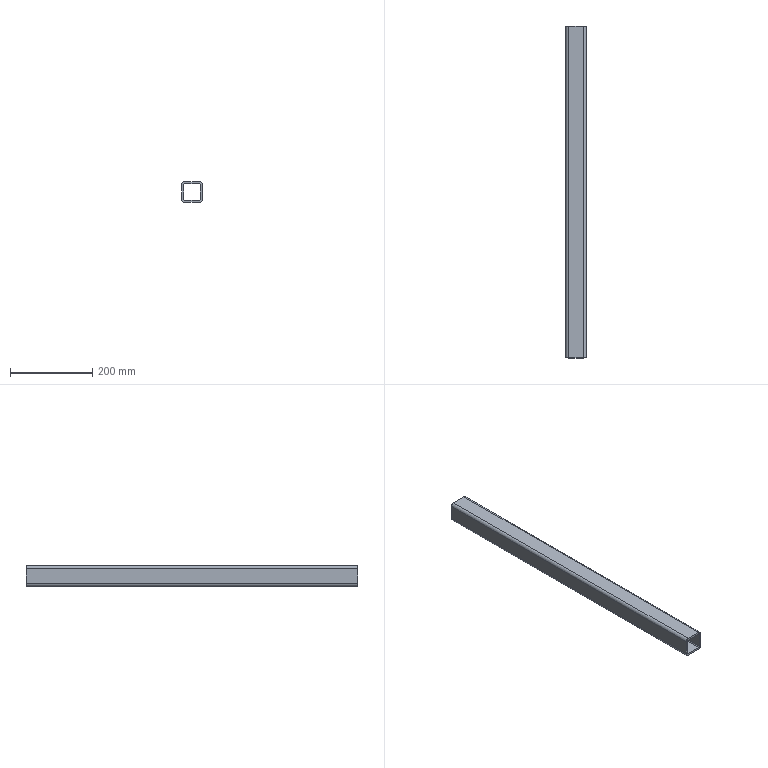Part | NX | 1 solid | 21 faces | box 50 x 806 x 50 mm | volume 694058 mm3 | cylinder 11 | plane 10 | commonest cylinder face diameters 4 x4 14 x4 4.2 x3
STEP:
#1=CARTESIAN_POINT('',(-895.,25.,-328.));
#2=VERTEX_POINT('',#1);
#3=CARTESIAN_POINT('',(-895.,831.,-328.));
#4=VERTEX_POINT('',#3);
#5=CARTESIAN_POINT('',(-895.,0.,-328.));
#6=DIRECTION('',(0.,1.,0.));
#7=VECTOR('',#6,1000.);
#8=LINE('',#5,#7);
#9=EDGE_CURVE('',#2,#4,#8,.T.);
#10=ORIENTED_EDGE('',*,*,#9,.T.);
#11=CARTESIAN_POINT('',(-895.,831.,-292.));
#12=VERTEX_POINT('',#11);
#13=CARTESIAN_POINT('',(-895.,831.,-328.));
#14=DIRECTION('',(0.,0.,1.));
#15=VECTOR('',#14,1000.);
#16=LINE('',#13,#15);
#17=EDGE_CURVE('',#4,#12,#16,.T.);
#18=ORIENTED_EDGE('',*,*,#17,.T.);
#19=CARTESIAN_POINT('',(-895.,25.,-292.));
#20=VERTEX_POINT('',#19);
#21=CARTESIAN_POINT('',(-895.,0.,-292.));
#22=DIRECTION('',(0.,1.,0.));
#23=VECTOR('',#22,1000.);
#24=LINE('',#21,#23);
#25=EDGE_CURVE('',#20,#12,#24,.T.);
#26=ORIENTED_EDGE('',*,*,#25,.F.);
#27=CARTESIAN_POINT('',(-895.,25.,-328.));
#28=DIRECTION('',(0.,0.,-1.));
#29=VECTOR('',#28,1000.);
#30=LINE('',#27,#29);
#31=EDGE_CURVE('',#20,#2,#30,.T.);
#32=ORIENTED_EDGE('',*,*,#31,.T.);
#33=EDGE_LOOP('',(#10,#18,#26,#32));
#34=FACE_BOUND('',#33,.T.);
#35=CARTESIAN_POINT('',(-895.,0.,-328.));
#36=DIRECTION('',(1.,0.,0.));
#37=DIRECTION('',(0.,0.,-1.));
#38=AXIS2_PLACEMENT_3D('',#35,#36,#37);
#39=PLANE('',#38);
#40=ADVANCED_FACE('',(#34),#39,.T.);
#41=CARTESIAN_POINT('',(-893.,25.,-330.));
#42=VERTEX_POINT('',#41);
#43=CARTESIAN_POINT('',(-893.,831.,-330.));
#44=VERTEX_POINT('',#43);
#45=CARTESIAN_POINT('',(-893.,0.,-330.));
#46=DIRECTION('',(0.,1.,0.));
#47=VECTOR('',#46,1000.);
#48=LINE('',#45,#47);
#49=EDGE_CURVE('',#42,#44,#48,.T.);
#50=ORIENTED_EDGE('',*,*,#49,.T.);
#51=CARTESIAN_POINT('',(-893.,831.,-328.));
#52=DIRECTION('',(0.,1.,0.));
#53=DIRECTION('',(-1.,0.,0.));
#54=AXIS2_PLACEMENT_3D('',#51,#52,#53);
#55=CIRCLE('',#54,2.);
#56=EDGE_CURVE('',#44,#4,#55,.T.);
#57=ORIENTED_EDGE('',*,*,#56,.T.);
#58=ORIENTED_EDGE('',*,*,#9,.F.);
#59=CARTESIAN_POINT('',(-893.,25.,-328.));
#60=DIRECTION('',(0.,-1.,0.));
#61=DIRECTION('',(1.,0.,0.));
#62=AXIS2_PLACEMENT_3D('',#59,#60,#61);
#63=CIRCLE('',#62,2.);
#64=EDGE_CURVE('',#2,#42,#63,.T.);
#65=ORIENTED_EDGE('',*,*,#64,.T.);
#66=EDGE_LOOP('',(#50,#57,#58,#65));
#67=FACE_BOUND('',#66,.T.);
#68=CARTESIAN_POINT('',(-893.,0.,-328.));
#69=DIRECTION('',(0.,1.,0.));
#70=DIRECTION('',(0.,0.,1.));
#71=AXIS2_PLACEMENT_3D('',#68,#69,#70);
#72=CYLINDRICAL_SURFACE('',#71,2.);
#73=ADVANCED_FACE('',(#67),#72,.F.);
#74=CARTESIAN_POINT('',(-857.,25.,-330.));
#75=VERTEX_POINT('',#74);
#76=CARTESIAN_POINT('',(-857.,831.,-330.));
#77=VERTEX_POINT('',#76);
#78=CARTESIAN_POINT('',(-857.,0.,-330.));
#79=DIRECTION('',(0.,1.,0.));
#80=VECTOR('',#79,1000.);
#81=LINE('',#78,#80);
#82=EDGE_CURVE('',#75,#77,#81,.T.);
#83=ORIENTED_EDGE('',*,*,#82,.T.);
#84=CARTESIAN_POINT('',(-893.,831.,-330.));
#85=DIRECTION('',(-1.,0.,0.));
#86=VECTOR('',#85,1000.);
#87=LINE('',#84,#86);
#88=EDGE_CURVE('',#77,#44,#87,.T.);
#89=ORIENTED_EDGE('',*,*,#88,.T.);
#90=ORIENTED_EDGE('',*,*,#49,.F.);
#91=CARTESIAN_POINT('',(-893.,25.,-330.));
#92=DIRECTION('',(1.,0.,0.));
#93=VECTOR('',#92,1000.);
#94=LINE('',#91,#93);
#95=EDGE_CURVE('',#42,#75,#94,.T.);
#96=ORIENTED_EDGE('',*,*,#95,.T.);
#97=EDGE_LOOP('',(#83,#89,#90,#96));
#98=FACE_BOUND('',#97,.T.);
#99=CARTESIAN_POINT('',(-893.,0.,-330.));
#100=DIRECTION('',(0.,0.,1.));
#101=DIRECTION('',(1.,0.,0.));
#102=AXIS2_PLACEMENT_3D('',#99,#100,#101);
#103=PLANE('',#102);
#104=ADVANCED_FACE('',(#98),#103,.T.);
#105=CARTESIAN_POINT('',(-855.,25.,-328.));
#106=VERTEX_POINT('',#105);
#107=CARTESIAN_POINT('',(-855.,831.,-328.));
#108=VERTEX_POINT('',#107);
#109=CARTESIAN_POINT('',(-855.,0.,-328.));
#110=DIRECTION('',(0.,1.,0.));
#111=VECTOR('',#110,1000.);
#112=LINE('',#109,#111);
#113=EDGE_CURVE('',#106,#108,#112,.T.);
#114=ORIENTED_EDGE('',*,*,#113,.T.);
#115=CARTESIAN_POINT('',(-857.,831.,-328.));
#116=DIRECTION('',(0.,1.,0.));
#117=DIRECTION('',(-1.,0.,0.));
#118=AXIS2_PLACEMENT_3D('',#115,#116,#117);
#119=CIRCLE('',#118,2.);
#120=EDGE_CURVE('',#108,#77,#119,.T.);
#121=ORIENTED_EDGE('',*,*,#120,.T.);
#122=ORIENTED_EDGE('',*,*,#82,.F.);
#123=CARTESIAN_POINT('',(-857.,25.,-328.));
#124=DIRECTION('',(0.,-1.,0.));
#125=DIRECTION('',(1.,0.,0.));
#126=AXIS2_PLACEMENT_3D('',#123,#124,#125);
#127=CIRCLE('',#126,2.);
#128=EDGE_CURVE('',#75,#106,#127,.T.);
#129=ORIENTED_EDGE('',*,*,#128,.T.);
#130=EDGE_LOOP('',(#114,#121,#122,#129));
#131=FACE_BOUND('',#130,.T.);
#132=CARTESIAN_POINT('',(-857.,0.,-328.));
#133=DIRECTION('',(0.,1.,0.));
#134=DIRECTION('',(0.,0.,1.));
#135=AXIS2_PLACEMENT_3D('',#132,#133,#134);
#136=CYLINDRICAL_SURFACE('',#135,2.);
#137=ADVANCED_FACE('',(#131),#136,.F.);
#138=CARTESIAN_POINT('',(-855.,131.,-307.9));
#139=VERTEX_POINT('',#138);
#140=CARTESIAN_POINT('',(-855.,131.,-310.));
#141=DIRECTION('',(-1.,0.,0.));
#142=DIRECTION('',(0.,0.,1.));
#143=AXIS2_PLACEMENT_3D('',#140,#141,#142);
#144=CIRCLE('',#143,2.1);
#145=EDGE_CURVE('',#139,#139,#144,.T.);
#146=ORIENTED_EDGE('',*,*,#145,.F.);
#147=EDGE_LOOP('',(#146));
#148=FACE_BOUND('',#147,.T.);
#149=CARTESIAN_POINT('',(-855.,431.,-307.9));
#150=VERTEX_POINT('',#149);
#151=CARTESIAN_POINT('',(-855.,431.,-310.));
#152=DIRECTION('',(-1.,0.,0.));
#153=DIRECTION('',(0.,0.,1.));
#154=AXIS2_PLACEMENT_3D('',#151,#152,#153);
#155=CIRCLE('',#154,2.1);
#156=EDGE_CURVE('',#150,#150,#155,.T.);
#157=ORIENTED_EDGE('',*,*,#156,.F.);
#158=EDGE_LOOP('',(#157));
#159=FACE_BOUND('',#158,.T.);
#160=CARTESIAN_POINT('',(-855.,731.,-307.9));
#161=VERTEX_POINT('',#160);
#162=CARTESIAN_POINT('',(-855.,731.,-310.));
#163=DIRECTION('',(-1.,0.,0.));
#164=DIRECTION('',(0.,0.,1.));
#165=AXIS2_PLACEMENT_3D('',#162,#163,#164);
#166=CIRCLE('',#165,2.1);
#167=EDGE_CURVE('',#161,#161,#166,.T.);
#168=ORIENTED_EDGE('',*,*,#167,.F.);
#169=EDGE_LOOP('',(#168));
#170=FACE_BOUND('',#169,.T.);
#171=CARTESIAN_POINT('',(-855.,25.,-292.));
#172=VERTEX_POINT('',#171);
#173=CARTESIAN_POINT('',(-855.,831.,-292.));
#174=VERTEX_POINT('',#173);
#175=CARTESIAN_POINT('',(-855.,0.,-292.));
#176=DIRECTION('',(0.,1.,0.));
#177=VECTOR('',#176,1000.);
#178=LINE('',#175,#177);
#179=EDGE_CURVE('',#172,#174,#178,.T.);
#180=ORIENTED_EDGE('',*,*,#179,.T.);
#181=CARTESIAN_POINT('',(-855.,831.,-292.));
#182=DIRECTION('',(0.,0.,-1.));
#183=VECTOR('',#182,1000.);
#184=LINE('',#181,#183);
#185=EDGE_CURVE('',#174,#108,#184,.T.);
#186=ORIENTED_EDGE('',*,*,#185,.T.);
#187=ORIENTED_EDGE('',*,*,#113,.F.);
#188=CARTESIAN_POINT('',(-855.,25.,-292.));
#189=DIRECTION('',(0.,0.,1.));
#190=VECTOR('',#189,1000.);
#191=LINE('',#188,#190);
#192=EDGE_CURVE('',#106,#172,#191,.T.);
#193=ORIENTED_EDGE('',*,*,#192,.T.);
#194=EDGE_LOOP('',(#180,#186,#187,#193));
#195=FACE_BOUND('',#194,.T.);
#196=CARTESIAN_POINT('',(-855.,0.,-292.));
#197=DIRECTION('',(-1.,0.,0.));
#198=DIRECTION('',(0.,0.,1.));
#199=AXIS2_PLACEMENT_3D('',#196,#197,#198);
#200=PLANE('',#199);
#201=ADVANCED_FACE('',(#148,#159,#170,#195),#200,.T.);
#202=CARTESIAN_POINT('',(-857.,25.,-290.));
#203=VERTEX_POINT('',#202);
#204=CARTESIAN_POINT('',(-857.,831.,-290.));
#205=VERTEX_POINT('',#204);
#206=CARTESIAN_POINT('',(-857.,0.,-290.));
#207=DIRECTION('',(0.,1.,0.));
#208=VECTOR('',#207,1000.);
#209=LINE('',#206,#208);
#210=EDGE_CURVE('',#203,#205,#209,.T.);
#211=ORIENTED_EDGE('',*,*,#210,.T.);
#212=CARTESIAN_POINT('',(-857.,831.,-292.));
#213=DIRECTION('',(0.,1.,0.));
#214=DIRECTION('',(-1.,0.,0.));
#215=AXIS2_PLACEMENT_3D('',#212,#213,#214);
#216=CIRCLE('',#215,2.);
#217=EDGE_CURVE('',#205,#174,#216,.T.);
#218=ORIENTED_EDGE('',*,*,#217,.T.);
#219=ORIENTED_EDGE('',*,*,#179,.F.);
#220=CARTESIAN_POINT('',(-857.,25.,-292.));
#221=DIRECTION('',(0.,-1.,0.));
#222=DIRECTION('',(1.,0.,0.));
#223=AXIS2_PLACEMENT_3D('',#220,#221,#222);
#224=CIRCLE('',#223,2.);
#225=EDGE_CURVE('',#172,#203,#224,.T.);
#226=ORIENTED_EDGE('',*,*,#225,.T.);
#227=EDGE_LOOP('',(#211,#218,#219,#226));
#228=FACE_BOUND('',#227,.T.);
#229=CARTESIAN_POINT('',(-857.,0.,-292.));
#230=DIRECTION('',(0.,1.,0.));
#231=DIRECTION('',(0.,0.,1.));
#232=AXIS2_PLACEMENT_3D('',#229,#230,#231);
#233=CYLINDRICAL_SURFACE('',#232,2.);
#234=ADVANCED_FACE('',(#228),#233,.F.);
#235=CARTESIAN_POINT('',(-893.,25.,-290.));
#236=VERTEX_POINT('',#235);
#237=CARTESIAN_POINT('',(-893.,831.,-290.));
#238=VERTEX_POINT('',#237);
#239=CARTESIAN_POINT('',(-893.,0.,-290.));
#240=DIRECTION('',(0.,1.,0.));
#241=VECTOR('',#240,1000.);
#242=LINE('',#239,#241);
#243=EDGE_CURVE('',#236,#238,#242,.T.);
#244=ORIENTED_EDGE('',*,*,#243,.T.);
#245=CARTESIAN_POINT('',(-857.,831.,-290.));
#246=DIRECTION('',(1.,0.,0.));
#247=VECTOR('',#246,1000.);
#248=LINE('',#245,#247);
#249=EDGE_CURVE('',#238,#205,#248,.T.);
#250=ORIENTED_EDGE('',*,*,#249,.T.);
#251=ORIENTED_EDGE('',*,*,#210,.F.);
#252=CARTESIAN_POINT('',(-857.,25.,-290.));
#253=DIRECTION('',(-1.,0.,0.));
#254=VECTOR('',#253,1000.);
#255=LINE('',#252,#254);
#256=EDGE_CURVE('',#203,#236,#255,.T.);
#257=ORIENTED_EDGE('',*,*,#256,.T.);
#258=EDGE_LOOP('',(#244,#250,#251,#257));
#259=FACE_BOUND('',#258,.T.);
#260=CARTESIAN_POINT('',(-857.,0.,-290.));
#261=DIRECTION('',(0.,0.,-1.));
#262=DIRECTION('',(-1.,0.,0.));
#263=AXIS2_PLACEMENT_3D('',#260,#261,#262);
#264=PLANE('',#263);
#265=ADVANCED_FACE('',(#259),#264,.T.);
#266=ORIENTED_EDGE('',*,*,#25,.T.);
#267=CARTESIAN_POINT('',(-893.,831.,-292.));
#268=DIRECTION('',(0.,1.,0.));
#269=DIRECTION('',(-1.,0.,0.));
#270=AXIS2_PLACEMENT_3D('',#267,#268,#269);
#271=CIRCLE('',#270,2.);
#272=EDGE_CURVE('',#12,#238,#271,.T.);
#273=ORIENTED_EDGE('',*,*,#272,.T.);
#274=ORIENTED_EDGE('',*,*,#243,.F.);
#275=CARTESIAN_POINT('',(-893.,25.,-292.));
#276=DIRECTION('',(0.,-1.,0.));
#277=DIRECTION('',(1.,0.,0.));
#278=AXIS2_PLACEMENT_3D('',#275,#276,#277);
#279=CIRCLE('',#278,2.);
#280=EDGE_CURVE('',#236,#20,#279,.T.);
#281=ORIENTED_EDGE('',*,*,#280,.T.);
#282=EDGE_LOOP('',(#266,#273,#274,#281));
#283=FACE_BOUND('',#282,.T.);
#284=CARTESIAN_POINT('',(-893.,0.,-292.));
#285=DIRECTION('',(0.,1.,0.));
#286=DIRECTION('',(0.,0.,1.));
#287=AXIS2_PLACEMENT_3D('',#284,#285,#286);
#288=CYLINDRICAL_SURFACE('',#287,2.);
#289=ADVANCED_FACE('',(#283),#288,.F.);
#290=CARTESIAN_POINT('',(-850.,131.,-312.1));
#291=VERTEX_POINT('',#290);
#292=CARTESIAN_POINT('',(-850.,131.,-310.));
#293=DIRECTION('',(1.,0.,0.));
#294=DIRECTION('',(0.,0.,-1.));
#295=AXIS2_PLACEMENT_3D('',#292,#293,#294);
#296=CIRCLE('',#295,2.1);
#297=EDGE_CURVE('',#291,#291,#296,.T.);
#298=ORIENTED_EDGE('',*,*,#297,.F.);
#299=EDGE_LOOP('',(#298));
#300=FACE_BOUND('',#299,.T.);
#301=CARTESIAN_POINT('',(-850.,431.,-312.1));
#302=VERTEX_POINT('',#301);
#303=CARTESIAN_POINT('',(-850.,431.,-310.));
#304=DIRECTION('',(1.,0.,0.));
#305=DIRECTION('',(0.,0.,-1.));
#306=AXIS2_PLACEMENT_3D('',#303,#304,#305);
#307=CIRCLE('',#306,2.1);
#308=EDGE_CURVE('',#302,#302,#307,.T.);
#309=ORIENTED_EDGE('',*,*,#308,.F.);
#310=EDGE_LOOP('',(#309));
#311=FACE_BOUND('',#310,.T.);
#312=CARTESIAN_POINT('',(-850.,731.,-312.1));
#313=VERTEX_POINT('',#312);
#314=CARTESIAN_POINT('',(-850.,731.,-310.));
#315=DIRECTION('',(1.,0.,0.));
#316=DIRECTION('',(0.,0.,-1.));
#317=AXIS2_PLACEMENT_3D('',#314,#315,#316);
#318=CIRCLE('',#317,2.1);
#319=EDGE_CURVE('',#313,#313,#318,.T.);
#320=ORIENTED_EDGE('',*,*,#319,.F.);
#321=EDGE_LOOP('',(#320));
#322=FACE_BOUND('',#321,.T.);
#323=CARTESIAN_POINT('',(-850.,831.,-292.));
#324=VERTEX_POINT('',#323);
#325=CARTESIAN_POINT('',(-850.,831.,-328.));
#326=VERTEX_POINT('',#325);
#327=CARTESIAN_POINT('',(-850.,831.,350.));
#328=DIRECTION('',(0.,0.,-1.));
#329=VECTOR('',#328,1000.);
#330=LINE('',#327,#329);
#331=EDGE_CURVE('',#324,#326,#330,.T.);
#332=ORIENTED_EDGE('',*,*,#331,.F.);
#333=CARTESIAN_POINT('',(-850.,25.,-292.));
#334=VERTEX_POINT('',#333);
#335=CARTESIAN_POINT('',(-850.,0.,-292.));
#336=DIRECTION('',(0.,1.,0.));
#337=VECTOR('',#336,1000.);
#338=LINE('',#335,#337);
#339=EDGE_CURVE('',#334,#324,#338,.T.);
#340=ORIENTED_EDGE('',*,*,#339,.F.);
#341=CARTESIAN_POINT('',(-850.,25.,-328.));
#342=VERTEX_POINT('',#341);
#343=CARTESIAN_POINT('',(-850.,25.,-292.));
#344=DIRECTION('',(0.,0.,1.));
#345=VECTOR('',#344,1000.);
#346=LINE('',#343,#345);
#347=EDGE_CURVE('',#342,#334,#346,.T.);
#348=ORIENTED_EDGE('',*,*,#347,.F.);
#349=CARTESIAN_POINT('',(-850.,0.,-328.));
#350=DIRECTION('',(0.,1.,0.));
#351=VECTOR('',#350,1000.);
#352=LINE('',#349,#351);
#353=EDGE_CURVE('',#342,#326,#352,.T.);
#354=ORIENTED_EDGE('',*,*,#353,.T.);
#355=EDGE_LOOP('',(#332,#340,#348,#354));
#356=FACE_BOUND('',#355,.T.);
#357=CARTESIAN_POINT('',(-850.,0.,-292.));
#358=DIRECTION('',(-1.,0.,0.));
#359=DIRECTION('',(0.,0.,1.));
#360=AXIS2_PLACEMENT_3D('',#357,#358,#359);
#361=PLANE('',#360);
#362=ADVANCED_FACE('',(#300,#311,#322,#356),#361,.F.);
#363=CARTESIAN_POINT('',(-857.,831.,-335.));
#364=VERTEX_POINT('',#363);
#365=CARTESIAN_POINT('',(-857.,831.,-328.));
#366=DIRECTION('',(0.,1.,0.));
#367=DIRECTION('',(-1.,0.,0.));
#368=AXIS2_PLACEMENT_3D('',#365,#366,#367);
#369=CIRCLE('',#368,7.);
#370=EDGE_CURVE('',#326,#364,#369,.T.);
#371=ORIENTED_EDGE('',*,*,#370,.F.);
#372=ORIENTED_EDGE('',*,*,#353,.F.);
#373=CARTESIAN_POINT('',(-857.,25.,-335.));
#374=VERTEX_POINT('',#373);
#375=CARTESIAN_POINT('',(-857.,25.,-328.));
#376=DIRECTION('',(0.,-1.,0.));
#377=DIRECTION('',(1.,0.,0.));
#378=AXIS2_PLACEMENT_3D('',#375,#376,#377);
#379=CIRCLE('',#378,7.);
#380=EDGE_CURVE('',#374,#342,#379,.T.);
#381=ORIENTED_EDGE('',*,*,#380,.F.);
#382=CARTESIAN_POINT('',(-857.,0.,-335.));
#383=DIRECTION('',(0.,1.,0.));
#384=VECTOR('',#383,1000.);
#385=LINE('',#382,#384);
#386=EDGE_CURVE('',#374,#364,#385,.T.);
#387=ORIENTED_EDGE('',*,*,#386,.T.);
#388=EDGE_LOOP('',(#371,#372,#381,#387));
#389=FACE_BOUND('',#388,.T.);
#390=CARTESIAN_POINT('',(-857.,0.,-328.));
#391=DIRECTION('',(0.,1.,0.));
#392=DIRECTION('',(0.,0.,1.));
#393=AXIS2_PLACEMENT_3D('',#390,#391,#392);
#394=CYLINDRICAL_SURFACE('',#393,7.);
#395=ADVANCED_FACE('',(#389),#394,.T.);
#396=CARTESIAN_POINT('',(-893.,831.,-335.));
#397=VERTEX_POINT('',#396);
#398=CARTESIAN_POINT('',(-893.,831.,-335.));
#399=DIRECTION('',(-1.,0.,0.));
#400=VECTOR('',#399,1000.);
#401=LINE('',#398,#400);
#402=EDGE_CURVE('',#364,#397,#401,.T.);
#403=ORIENTED_EDGE('',*,*,#402,.F.);
#404=ORIENTED_EDGE('',*,*,#386,.F.);
#405=CARTESIAN_POINT('',(-893.,25.,-335.));
#406=VERTEX_POINT('',#405);
#407=CARTESIAN_POINT('',(-893.,25.,-335.));
#408=DIRECTION('',(1.,0.,0.));
#409=VECTOR('',#408,1000.);
#410=LINE('',#407,#409);
#411=EDGE_CURVE('',#406,#374,#410,.T.);
#412=ORIENTED_EDGE('',*,*,#411,.F.);
#413=CARTESIAN_POINT('',(-893.,0.,-335.));
#414=DIRECTION('',(0.,1.,0.));
#415=VECTOR('',#414,1000.);
#416=LINE('',#413,#415);
#417=EDGE_CURVE('',#406,#397,#416,.T.);
#418=ORIENTED_EDGE('',*,*,#417,.T.);
#419=EDGE_LOOP('',(#403,#404,#412,#418));
#420=FACE_BOUND('',#419,.T.);
#421=CARTESIAN_POINT('',(-893.,0.,-335.));
#422=DIRECTION('',(0.,0.,1.));
#423=DIRECTION('',(1.,0.,0.));
#424=AXIS2_PLACEMENT_3D('',#421,#422,#423);
#425=PLANE('',#424);
#426=ADVANCED_FACE('',(#420),#425,.F.);
#427=CARTESIAN_POINT('',(-900.,831.,-328.));
#428=VERTEX_POINT('',#427);
#429=CARTESIAN_POINT('',(-893.,831.,-328.));
#430=DIRECTION('',(0.,1.,0.));
#431=DIRECTION('',(-1.,0.,0.));
#432=AXIS2_PLACEMENT_3D('',#429,#430,#431);
#433=CIRCLE('',#432,7.);
#434=EDGE_CURVE('',#397,#428,#433,.T.);
#435=ORIENTED_EDGE('',*,*,#434,.F.);
#436=ORIENTED_EDGE('',*,*,#417,.F.);
#437=CARTESIAN_POINT('',(-900.,25.,-328.));
#438=VERTEX_POINT('',#437);
#439=CARTESIAN_POINT('',(-893.,25.,-328.));
#440=DIRECTION('',(0.,-1.,0.));
#441=DIRECTION('',(1.,0.,0.));
#442=AXIS2_PLACEMENT_3D('',#439,#440,#441);
#443=CIRCLE('',#442,7.);
#444=EDGE_CURVE('',#438,#406,#443,.T.);
#445=ORIENTED_EDGE('',*,*,#444,.F.);
#446=CARTESIAN_POINT('',(-900.,0.,-328.));
#447=DIRECTION('',(0.,1.,0.));
#448=VECTOR('',#447,1000.);
#449=LINE('',#446,#448);
#450=EDGE_CURVE('',#438,#428,#449,.T.);
#451=ORIENTED_EDGE('',*,*,#450,.T.);
#452=EDGE_LOOP('',(#435,#436,#445,#451));
#453=FACE_BOUND('',#452,.T.);
#454=CARTESIAN_POINT('',(-893.,0.,-328.));
#455=DIRECTION('',(0.,1.,0.));
#456=DIRECTION('',(0.,0.,1.));
#457=AXIS2_PLACEMENT_3D('',#454,#455,#456);
#458=CYLINDRICAL_SURFACE('',#457,7.);
#459=ADVANCED_FACE('',(#453),#458,.T.);
#460=CARTESIAN_POINT('',(-900.,831.,-292.));
#461=VERTEX_POINT('',#460);
#462=CARTESIAN_POINT('',(-900.,831.,350.));
#463=DIRECTION('',(0.,0.,-1.));
#464=VECTOR('',#463,1000.);
#465=LINE('',#462,#464);
#466=EDGE_CURVE('',#461,#428,#465,.T.);
#467=ORIENTED_EDGE('',*,*,#466,.T.);
#468=ORIENTED_EDGE('',*,*,#450,.F.);
#469=CARTESIAN_POINT('',(-900.,25.,-292.));
#470=VERTEX_POINT('',#469);
#471=CARTESIAN_POINT('',(-900.,25.,575.));
#472=DIRECTION('',(0.,0.,-1.));
#473=VECTOR('',#472,1000.);
#474=LINE('',#471,#473);
#475=EDGE_CURVE('',#470,#438,#474,.T.);
#476=ORIENTED_EDGE('',*,*,#475,.F.);
#477=CARTESIAN_POINT('',(-900.,0.,-292.));
#478=DIRECTION('',(0.,1.,0.));
#479=VECTOR('',#478,1000.);
#480=LINE('',#477,#479);
#481=EDGE_CURVE('',#470,#461,#480,.T.);
#482=ORIENTED_EDGE('',*,*,#481,.T.);
#483=EDGE_LOOP('',(#467,#468,#476,#482));
#484=FACE_BOUND('',#483,.T.);
#485=CARTESIAN_POINT('',(-900.,0.,-328.));
#486=DIRECTION('',(1.,0.,0.));
#487=DIRECTION('',(0.,0.,-1.));
#488=AXIS2_PLACEMENT_3D('',#485,#486,#487);
#489=PLANE('',#488);
#490=ADVANCED_FACE('',(#484),#489,.F.);
#491=CARTESIAN_POINT('',(-893.,831.,-285.));
#492=VERTEX_POINT('',#491);
#493=CARTESIAN_POINT('',(-893.,831.,-292.));
#494=DIRECTION('',(0.,1.,0.));
#495=DIRECTION('',(-1.,0.,0.));
#496=AXIS2_PLACEMENT_3D('',#493,#494,#495);
#497=CIRCLE('',#496,7.);
#498=EDGE_CURVE('',#461,#492,#497,.T.);
#499=ORIENTED_EDGE('',*,*,#498,.F.);
#500=ORIENTED_EDGE('',*,*,#481,.F.);
#501=CARTESIAN_POINT('',(-893.,25.,-285.));
#502=VERTEX_POINT('',#501);
#503=CARTESIAN_POINT('',(-893.,25.,-292.));
#504=DIRECTION('',(0.,-1.,0.));
#505=DIRECTION('',(1.,0.,0.));
#506=AXIS2_PLACEMENT_3D('',#503,#504,#505);
#507=CIRCLE('',#506,7.);
#508=EDGE_CURVE('',#502,#470,#507,.T.);
#509=ORIENTED_EDGE('',*,*,#508,.F.);
#510=CARTESIAN_POINT('',(-893.,0.,-285.));
#511=DIRECTION('',(0.,1.,0.));
#512=VECTOR('',#511,1000.);
#513=LINE('',#510,#512);
#514=EDGE_CURVE('',#502,#492,#513,.T.);
#515=ORIENTED_EDGE('',*,*,#514,.T.);
#516=EDGE_LOOP('',(#499,#500,#509,#515));
#517=FACE_BOUND('',#516,.T.);
#518=CARTESIAN_POINT('',(-893.,0.,-292.));
#519=DIRECTION('',(0.,1.,0.));
#520=DIRECTION('',(0.,0.,1.));
#521=AXIS2_PLACEMENT_3D('',#518,#519,#520);
#522=CYLINDRICAL_SURFACE('',#521,7.);
#523=ADVANCED_FACE('',(#517),#522,.T.);
#524=CARTESIAN_POINT('',(-857.,831.,-285.));
#525=VERTEX_POINT('',#524);
#526=CARTESIAN_POINT('',(-857.,831.,-285.));
#527=DIRECTION('',(1.,0.,0.));
#528=VECTOR('',#527,1000.);
#529=LINE('',#526,#528);
#530=EDGE_CURVE('',#492,#525,#529,.T.);
#531=ORIENTED_EDGE('',*,*,#530,.F.);
#532=ORIENTED_EDGE('',*,*,#514,.F.);
#533=CARTESIAN_POINT('',(-857.,25.,-285.));
#534=VERTEX_POINT('',#533);
#535=CARTESIAN_POINT('',(-857.,25.,-285.));
#536=DIRECTION('',(-1.,0.,0.));
#537=VECTOR('',#536,1000.);
#538=LINE('',#535,#537);
#539=EDGE_CURVE('',#534,#502,#538,.T.);
#540=ORIENTED_EDGE('',*,*,#539,.F.);
#541=CARTESIAN_POINT('',(-857.,0.,-285.));
#542=DIRECTION('',(0.,1.,0.));
#543=VECTOR('',#542,1000.);
#544=LINE('',#541,#543);
#545=EDGE_CURVE('',#534,#525,#544,.T.);
#546=ORIENTED_EDGE('',*,*,#545,.T.);
#547=EDGE_LOOP('',(#531,#532,#540,#546));
#548=FACE_BOUND('',#547,.T.);
#549=CARTESIAN_POINT('',(-857.,0.,-285.));
#550=DIRECTION('',(0.,0.,-1.));
#551=DIRECTION('',(-1.,0.,0.));
#552=AXIS2_PLACEMENT_3D('',#549,#550,#551);
#553=PLANE('',#552);
#554=ADVANCED_FACE('',(#548),#553,.F.);
#555=CARTESIAN_POINT('',(-857.,831.,-292.));
#556=DIRECTION('',(0.,1.,0.));
#557=DIRECTION('',(-1.,0.,0.));
#558=AXIS2_PLACEMENT_3D('',#555,#556,#557);
#559=CIRCLE('',#558,7.);
#560=EDGE_CURVE('',#525,#324,#559,.T.);
#561=ORIENTED_EDGE('',*,*,#560,.F.);
#562=ORIENTED_EDGE('',*,*,#545,.F.);
#563=CARTESIAN_POINT('',(-857.,25.,-292.));
#564=DIRECTION('',(0.,-1.,0.));
#565=DIRECTION('',(1.,0.,0.));
#566=AXIS2_PLACEMENT_3D('',#563,#564,#565);
#567=CIRCLE('',#566,7.);
#568=EDGE_CURVE('',#334,#534,#567,.T.);
#569=ORIENTED_EDGE('',*,*,#568,.F.);
#570=ORIENTED_EDGE('',*,*,#339,.T.);
#571=EDGE_LOOP('',(#561,#562,#569,#570));
#572=FACE_BOUND('',#571,.T.);
#573=CARTESIAN_POINT('',(-857.,0.,-292.));
#574=DIRECTION('',(0.,1.,0.));
#575=DIRECTION('',(0.,0.,1.));
#576=AXIS2_PLACEMENT_3D('',#573,#574,#575);
#577=CYLINDRICAL_SURFACE('',#576,7.);
#578=ADVANCED_FACE('',(#572),#577,.T.);
#579=ORIENTED_EDGE('',*,*,#256,.F.);
#580=ORIENTED_EDGE('',*,*,#225,.F.);
#581=ORIENTED_EDGE('',*,*,#192,.F.);
#582=ORIENTED_EDGE('',*,*,#128,.F.);
#583=ORIENTED_EDGE('',*,*,#95,.F.);
#584=ORIENTED_EDGE('',*,*,#64,.F.);
#585=ORIENTED_EDGE('',*,*,#31,.F.);
#586=ORIENTED_EDGE('',*,*,#280,.F.);
#587=EDGE_LOOP('',(#579,#580,#581,#582,#583,#584,#585,#586));
#588=FACE_BOUND('',#587,.T.);
#589=ORIENTED_EDGE('',*,*,#568,.T.);
#590=ORIENTED_EDGE('',*,*,#539,.T.);
#591=ORIENTED_EDGE('',*,*,#508,.T.);
#592=ORIENTED_EDGE('',*,*,#475,.T.);
#593=ORIENTED_EDGE('',*,*,#444,.T.);
#594=ORIENTED_EDGE('',*,*,#411,.T.);
#595=ORIENTED_EDGE('',*,*,#380,.T.);
#596=ORIENTED_EDGE('',*,*,#347,.T.);
#597=EDGE_LOOP('',(#589,#590,#591,#592,#593,#594,#595,#596));
#598=FACE_BOUND('',#597,.T.);
#599=CARTESIAN_POINT('',(-857.,25.,575.));
#600=DIRECTION('',(0.,-1.,0.));
#601=DIRECTION('',(1.,0.,0.));
#602=AXIS2_PLACEMENT_3D('',#599,#600,#601);
#603=PLANE('',#602);
#604=ADVANCED_FACE('',(#588,#598),#603,.T.);
#605=ORIENTED_EDGE('',*,*,#56,.F.);
#606=ORIENTED_EDGE('',*,*,#88,.F.);
#607=ORIENTED_EDGE('',*,*,#120,.F.);
#608=ORIENTED_EDGE('',*,*,#185,.F.);
#609=ORIENTED_EDGE('',*,*,#217,.F.);
#610=ORIENTED_EDGE('',*,*,#249,.F.);
#611=ORIENTED_EDGE('',*,*,#272,.F.);
#612=ORIENTED_EDGE('',*,*,#17,.F.);
#613=EDGE_LOOP('',(#605,#606,#607,#608,#609,#610,#611,#612));
#614=FACE_BOUND('',#613,.T.);
#615=ORIENTED_EDGE('',*,*,#370,.T.);
#616=ORIENTED_EDGE('',*,*,#402,.T.);
#617=ORIENTED_EDGE('',*,*,#434,.T.);
#618=ORIENTED_EDGE('',*,*,#466,.F.);
#619=ORIENTED_EDGE('',*,*,#498,.T.);
#620=ORIENTED_EDGE('',*,*,#530,.T.);
#621=ORIENTED_EDGE('',*,*,#560,.T.);
#622=ORIENTED_EDGE('',*,*,#331,.T.);
#623=EDGE_LOOP('',(#615,#616,#617,#618,#619,#620,#621,#622));
#624=FACE_BOUND('',#623,.T.);
#625=CARTESIAN_POINT('',(-893.,831.,350.));
#626=DIRECTION('',(0.,1.,0.));
#627=DIRECTION('',(-1.,0.,0.));
#628=AXIS2_PLACEMENT_3D('',#625,#626,#627);
#629=PLANE('',#628);
#630=ADVANCED_FACE('',(#614,#624),#629,.T.);
#631=ORIENTED_EDGE('',*,*,#167,.T.);
#632=EDGE_LOOP('',(#631));
#633=FACE_BOUND('',#632,.T.);
#634=ORIENTED_EDGE('',*,*,#319,.T.);
#635=EDGE_LOOP('',(#634));
#636=FACE_BOUND('',#635,.T.);
#637=CARTESIAN_POINT('',(-850.,731.,-310.));
#638=DIRECTION('',(1.,0.,0.));
#639=DIRECTION('',(0.,0.,-1.));
#640=AXIS2_PLACEMENT_3D('',#637,#638,#639);
#641=CYLINDRICAL_SURFACE('',#640,2.1);
#642=ADVANCED_FACE('',(#633,#636),#641,.F.);
#643=ORIENTED_EDGE('',*,*,#156,.T.);
#644=EDGE_LOOP('',(#643));
#645=FACE_BOUND('',#644,.T.);
#646=ORIENTED_EDGE('',*,*,#308,.T.);
#647=EDGE_LOOP('',(#646));
#648=FACE_BOUND('',#647,.T.);
#649=CARTESIAN_POINT('',(-850.,431.,-310.));
#650=DIRECTION('',(1.,0.,0.));
#651=DIRECTION('',(0.,0.,-1.));
#652=AXIS2_PLACEMENT_3D('',#649,#650,#651);
#653=CYLINDRICAL_SURFACE('',#652,2.1);
#654=ADVANCED_FACE('',(#645,#648),#653,.F.);
#655=ORIENTED_EDGE('',*,*,#145,.T.);
#656=EDGE_LOOP('',(#655));
#657=FACE_BOUND('',#656,.T.);
#658=ORIENTED_EDGE('',*,*,#297,.T.);
#659=EDGE_LOOP('',(#658));
#660=FACE_BOUND('',#659,.T.);
#661=CARTESIAN_POINT('',(-850.,131.,-310.));
#662=DIRECTION('',(1.,0.,0.));
#663=DIRECTION('',(0.,0.,-1.));
#664=AXIS2_PLACEMENT_3D('',#661,#662,#663);
#665=CYLINDRICAL_SURFACE('',#664,2.1);
#666=ADVANCED_FACE('',(#657,#660),#665,.F.);
#667=CLOSED_SHELL('',(#40,#73,#104,#137,#201,#234,#265,#289,#362,#395,#426,#459,#490,#523,#554,#578,#604,#630,#642,#654,#666));
#668=MANIFOLD_SOLID_BREP('',#667);
#669=(LENGTH_UNIT()NAMED_UNIT(*)SI_UNIT(.MILLI.,.METRE.));
#670=UNCERTAINTY_MEASURE_WITH_UNIT(LENGTH_MEASURE(0.00001),#669,'','');
#671=(NAMED_UNIT(*)PLANE_ANGLE_UNIT()SI_UNIT($,.RADIAN.));
#672=(NAMED_UNIT(*)SI_UNIT($,.STERADIAN.)SOLID_ANGLE_UNIT());
#673=(GEOMETRIC_REPRESENTATION_CONTEXT(3)GLOBAL_UNCERTAINTY_ASSIGNED_CONTEXT((#670))GLOBAL_UNIT_ASSIGNED_CONTEXT((#669,#671,#672))REPRESENTATION_CONTEXT('',''));
#674=ADVANCED_BREP_SHAPE_REPRESENTATION('',(#668),#673);